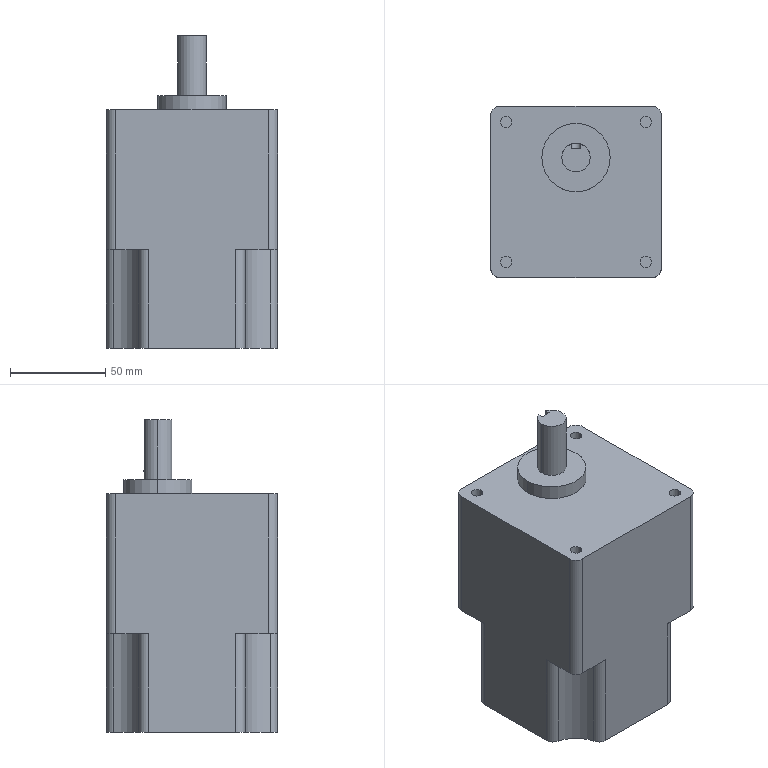Part | SolidWorks | features BaseBody 1 | 1 solid | 48 faces | box 90 x 90 x 164.5 mm | volume 974524 mm3 | cylinder 29 | plane 19 | commonest cylinder face diameters 10 x12 6 x8 35 x4 15 x2 36 x2 5 x1
STEP:
#1=CARTESIAN_POINT('',(-18.,18.,125.5));
#2=VERTEX_POINT('',#1);
#3=CARTESIAN_POINT('',(18.,18.,125.5));
#4=VERTEX_POINT('',#3);
#5=CARTESIAN_POINT('',(0.,18.,125.5));
#6=DIRECTION('',(0.,0.,-1.));
#7=DIRECTION('',(1.,0.,0.));
#8=AXIS2_PLACEMENT_3D('',#5,#6,#7);
#9=CIRCLE('',#8,18.);
#10=EDGE_CURVE('',#2,#4,#9,.T.);
#11=ORIENTED_EDGE('',*,*,#10,.F.);
#12=CARTESIAN_POINT('',(-18.,18.,133.));
#13=VERTEX_POINT('',#12);
#14=CARTESIAN_POINT('',(-18.,18.,125.5));
#15=DIRECTION('',(0.,0.,1.));
#16=VECTOR('',#15,1000.);
#17=LINE('',#14,#16);
#18=EDGE_CURVE('',#2,#13,#17,.T.);
#19=ORIENTED_EDGE('',*,*,#18,.T.);
#20=CARTESIAN_POINT('',(18.,18.,133.));
#21=VERTEX_POINT('',#20);
#22=CARTESIAN_POINT('',(0.,18.,133.));
#23=DIRECTION('',(0.,0.,-1.));
#24=DIRECTION('',(1.,0.,0.));
#25=AXIS2_PLACEMENT_3D('',#22,#23,#24);
#26=CIRCLE('',#25,18.);
#27=EDGE_CURVE('',#13,#21,#26,.T.);
#28=ORIENTED_EDGE('',*,*,#27,.T.);
#29=CARTESIAN_POINT('',(18.,18.,125.5));
#30=DIRECTION('',(0.,0.,1.));
#31=VECTOR('',#30,1000.);
#32=LINE('',#29,#31);
#33=EDGE_CURVE('',#4,#21,#32,.T.);
#34=ORIENTED_EDGE('',*,*,#33,.F.);
#35=EDGE_LOOP('',(#11,#19,#28,#34));
#36=FACE_OUTER_BOUND('',#35,.T.);
#37=CARTESIAN_POINT('',(0.,18.,125.5));
#38=DIRECTION('',(0.,0.,1.));
#39=DIRECTION('',(1.,0.,0.));
#40=AXIS2_PLACEMENT_3D('',#37,#38,#39);
#41=CYLINDRICAL_SURFACE('',#40,18.);
#42=ADVANCED_FACE('',(#36),#41,.T.);
#43=CARTESIAN_POINT('',(-39.77,36.77,110.5));
#44=VERTEX_POINT('',#43);
#45=CARTESIAN_POINT('',(-33.77,36.77,110.5));
#46=VERTEX_POINT('',#45);
#47=CARTESIAN_POINT('',(-36.77,36.77,110.5));
#48=DIRECTION('',(0.,0.,1.));
#49=DIRECTION('',(1.,0.,0.));
#50=AXIS2_PLACEMENT_3D('',#47,#48,#49);
#51=CIRCLE('',#50,3.);
#52=EDGE_CURVE('',#44,#46,#51,.T.);
#53=ORIENTED_EDGE('',*,*,#52,.F.);
#54=CARTESIAN_POINT('',(-39.77,36.77,125.5));
#55=VERTEX_POINT('',#54);
#56=CARTESIAN_POINT('',(-39.77,36.77,125.5));
#57=DIRECTION('',(0.,0.,1.));
#58=VECTOR('',#57,1000.);
#59=LINE('',#56,#58);
#60=EDGE_CURVE('',#44,#55,#59,.T.);
#61=ORIENTED_EDGE('',*,*,#60,.T.);
#62=CARTESIAN_POINT('',(-33.77,36.77,125.5));
#63=VERTEX_POINT('',#62);
#64=CARTESIAN_POINT('',(-36.77,36.77,125.5));
#65=DIRECTION('',(0.,0.,-1.));
#66=DIRECTION('',(1.,0.,0.));
#67=AXIS2_PLACEMENT_3D('',#64,#65,#66);
#68=CIRCLE('',#67,3.);
#69=EDGE_CURVE('',#63,#55,#68,.T.);
#70=ORIENTED_EDGE('',*,*,#69,.F.);
#71=CARTESIAN_POINT('',(-33.77,36.77,125.5));
#72=DIRECTION('',(0.,0.,1.));
#73=VECTOR('',#72,1000.);
#74=LINE('',#71,#73);
#75=EDGE_CURVE('',#46,#63,#74,.T.);
#76=ORIENTED_EDGE('',*,*,#75,.F.);
#77=EDGE_LOOP('',(#53,#61,#70,#76));
#78=FACE_OUTER_BOUND('',#77,.T.);
#79=CARTESIAN_POINT('',(-36.77,36.77,125.5));
#80=DIRECTION('',(0.,0.,1.));
#81=DIRECTION('',(1.,0.,0.));
#82=AXIS2_PLACEMENT_3D('',#79,#80,#81);
#83=CYLINDRICAL_SURFACE('',#82,3.);
#84=ADVANCED_FACE('',(#78),#83,.F.);
#85=CARTESIAN_POINT('',(33.77,36.77,110.5));
#86=VERTEX_POINT('',#85);
#87=CARTESIAN_POINT('',(39.77,36.77,110.5));
#88=VERTEX_POINT('',#87);
#89=CARTESIAN_POINT('',(36.77,36.77,110.5));
#90=DIRECTION('',(0.,0.,1.));
#91=DIRECTION('',(1.,0.,0.));
#92=AXIS2_PLACEMENT_3D('',#89,#90,#91);
#93=CIRCLE('',#92,3.);
#94=EDGE_CURVE('',#86,#88,#93,.T.);
#95=ORIENTED_EDGE('',*,*,#94,.F.);
#96=CARTESIAN_POINT('',(33.77,36.77,125.5));
#97=VERTEX_POINT('',#96);
#98=CARTESIAN_POINT('',(33.77,36.77,125.5));
#99=DIRECTION('',(0.,0.,1.));
#100=VECTOR('',#99,1000.);
#101=LINE('',#98,#100);
#102=EDGE_CURVE('',#86,#97,#101,.T.);
#103=ORIENTED_EDGE('',*,*,#102,.T.);
#104=CARTESIAN_POINT('',(39.77,36.77,125.5));
#105=VERTEX_POINT('',#104);
#106=CARTESIAN_POINT('',(36.77,36.77,125.5));
#107=DIRECTION('',(0.,0.,-1.));
#108=DIRECTION('',(1.,0.,0.));
#109=AXIS2_PLACEMENT_3D('',#106,#107,#108);
#110=CIRCLE('',#109,3.);
#111=EDGE_CURVE('',#105,#97,#110,.T.);
#112=ORIENTED_EDGE('',*,*,#111,.F.);
#113=CARTESIAN_POINT('',(39.77,36.77,125.5));
#114=DIRECTION('',(0.,0.,1.));
#115=VECTOR('',#114,1000.);
#116=LINE('',#113,#115);
#117=EDGE_CURVE('',#88,#105,#116,.T.);
#118=ORIENTED_EDGE('',*,*,#117,.F.);
#119=EDGE_LOOP('',(#95,#103,#112,#118));
#120=FACE_OUTER_BOUND('',#119,.T.);
#121=CARTESIAN_POINT('',(36.77,36.77,125.5));
#122=DIRECTION('',(0.,0.,1.));
#123=DIRECTION('',(1.,0.,0.));
#124=AXIS2_PLACEMENT_3D('',#121,#122,#123);
#125=CYLINDRICAL_SURFACE('',#124,3.);
#126=ADVANCED_FACE('',(#120),#125,.F.);
#127=CARTESIAN_POINT('',(33.77,-36.77,110.5));
#128=VERTEX_POINT('',#127);
#129=CARTESIAN_POINT('',(39.77,-36.77,110.5));
#130=VERTEX_POINT('',#129);
#131=CARTESIAN_POINT('',(36.77,-36.77,110.5));
#132=DIRECTION('',(0.,0.,1.));
#133=DIRECTION('',(1.,0.,0.));
#134=AXIS2_PLACEMENT_3D('',#131,#132,#133);
#135=CIRCLE('',#134,3.);
#136=EDGE_CURVE('',#128,#130,#135,.T.);
#137=ORIENTED_EDGE('',*,*,#136,.F.);
#138=CARTESIAN_POINT('',(33.77,-36.77,125.5));
#139=VERTEX_POINT('',#138);
#140=CARTESIAN_POINT('',(33.77,-36.77,125.5));
#141=DIRECTION('',(0.,0.,1.));
#142=VECTOR('',#141,1000.);
#143=LINE('',#140,#142);
#144=EDGE_CURVE('',#128,#139,#143,.T.);
#145=ORIENTED_EDGE('',*,*,#144,.T.);
#146=CARTESIAN_POINT('',(39.77,-36.77,125.5));
#147=VERTEX_POINT('',#146);
#148=CARTESIAN_POINT('',(36.77,-36.77,125.5));
#149=DIRECTION('',(0.,0.,-1.));
#150=DIRECTION('',(1.,0.,0.));
#151=AXIS2_PLACEMENT_3D('',#148,#149,#150);
#152=CIRCLE('',#151,3.);
#153=EDGE_CURVE('',#147,#139,#152,.T.);
#154=ORIENTED_EDGE('',*,*,#153,.F.);
#155=CARTESIAN_POINT('',(39.77,-36.77,125.5));
#156=DIRECTION('',(0.,0.,1.));
#157=VECTOR('',#156,1000.);
#158=LINE('',#155,#157);
#159=EDGE_CURVE('',#130,#147,#158,.T.);
#160=ORIENTED_EDGE('',*,*,#159,.F.);
#161=EDGE_LOOP('',(#137,#145,#154,#160));
#162=FACE_OUTER_BOUND('',#161,.T.);
#163=CARTESIAN_POINT('',(36.77,-36.77,125.5));
#164=DIRECTION('',(0.,0.,1.));
#165=DIRECTION('',(1.,0.,0.));
#166=AXIS2_PLACEMENT_3D('',#163,#164,#165);
#167=CYLINDRICAL_SURFACE('',#166,3.);
#168=ADVANCED_FACE('',(#162),#167,.F.);
#169=CARTESIAN_POINT('',(-39.77,-36.77,110.5));
#170=VERTEX_POINT('',#169);
#171=CARTESIAN_POINT('',(-33.77,-36.77,110.5));
#172=VERTEX_POINT('',#171);
#173=CARTESIAN_POINT('',(-36.77,-36.77,110.5));
#174=DIRECTION('',(0.,0.,1.));
#175=DIRECTION('',(1.,0.,0.));
#176=AXIS2_PLACEMENT_3D('',#173,#174,#175);
#177=CIRCLE('',#176,3.);
#178=EDGE_CURVE('',#170,#172,#177,.T.);
#179=ORIENTED_EDGE('',*,*,#178,.F.);
#180=CARTESIAN_POINT('',(-39.77,-36.77,125.5));
#181=VERTEX_POINT('',#180);
#182=CARTESIAN_POINT('',(-39.77,-36.77,125.5));
#183=DIRECTION('',(0.,0.,1.));
#184=VECTOR('',#183,1000.);
#185=LINE('',#182,#184);
#186=EDGE_CURVE('',#170,#181,#185,.T.);
#187=ORIENTED_EDGE('',*,*,#186,.T.);
#188=CARTESIAN_POINT('',(-33.77,-36.77,125.5));
#189=VERTEX_POINT('',#188);
#190=CARTESIAN_POINT('',(-36.77,-36.77,125.5));
#191=DIRECTION('',(0.,0.,-1.));
#192=DIRECTION('',(1.,0.,0.));
#193=AXIS2_PLACEMENT_3D('',#190,#191,#192);
#194=CIRCLE('',#193,3.);
#195=EDGE_CURVE('',#189,#181,#194,.T.);
#196=ORIENTED_EDGE('',*,*,#195,.F.);
#197=CARTESIAN_POINT('',(-33.77,-36.77,125.5));
#198=DIRECTION('',(0.,0.,1.));
#199=VECTOR('',#198,1000.);
#200=LINE('',#197,#199);
#201=EDGE_CURVE('',#172,#189,#200,.T.);
#202=ORIENTED_EDGE('',*,*,#201,.F.);
#203=EDGE_LOOP('',(#179,#187,#196,#202));
#204=FACE_OUTER_BOUND('',#203,.T.);
#205=CARTESIAN_POINT('',(-36.77,-36.77,125.5));
#206=DIRECTION('',(0.,0.,1.));
#207=DIRECTION('',(1.,0.,0.));
#208=AXIS2_PLACEMENT_3D('',#205,#206,#207);
#209=CYLINDRICAL_SURFACE('',#208,3.);
#210=ADVANCED_FACE('',(#204),#209,.F.);
#211=CARTESIAN_POINT('',(-7.5,18.,133.));
#212=VERTEX_POINT('',#211);
#213=CARTESIAN_POINT('',(7.5,18.,133.));
#214=VERTEX_POINT('',#213);
#215=CARTESIAN_POINT('',(0.,18.,133.));
#216=DIRECTION('',(0.,0.,-1.));
#217=DIRECTION('',(1.,0.,0.));
#218=AXIS2_PLACEMENT_3D('',#215,#216,#217);
#219=CIRCLE('',#218,7.5);
#220=EDGE_CURVE('',#212,#214,#219,.T.);
#221=ORIENTED_EDGE('',*,*,#220,.F.);
#222=CARTESIAN_POINT('',(-7.5,18.,164.5));
#223=VERTEX_POINT('',#222);
#224=CARTESIAN_POINT('',(-7.5,18.,133.));
#225=DIRECTION('',(0.,0.,1.));
#226=VECTOR('',#225,1000.);
#227=LINE('',#224,#226);
#228=EDGE_CURVE('',#212,#223,#227,.T.);
#229=ORIENTED_EDGE('',*,*,#228,.T.);
#230=CARTESIAN_POINT('',(-2.5,25.071,164.5));
#231=VERTEX_POINT('',#230);
#232=CARTESIAN_POINT('',(0.,18.,164.5));
#233=DIRECTION('',(0.,0.,-1.));
#234=DIRECTION('',(1.,0.,0.));
#235=AXIS2_PLACEMENT_3D('',#232,#233,#234);
#236=CIRCLE('',#235,7.5);
#237=EDGE_CURVE('',#223,#231,#236,.T.);
#238=ORIENTED_EDGE('',*,*,#237,.T.);
#239=CARTESIAN_POINT('',(-2.5,25.071,139.5));
#240=VERTEX_POINT('',#239);
#241=CARTESIAN_POINT('',(-2.5,25.071,133.));
#242=DIRECTION('',(0.,0.,-1.));
#243=VECTOR('',#242,1000.);
#244=LINE('',#241,#243);
#245=EDGE_CURVE('',#231,#240,#244,.T.);
#246=ORIENTED_EDGE('',*,*,#245,.T.);
#247=CARTESIAN_POINT('',(2.5,25.071,139.5));
#248=VERTEX_POINT('',#247);
#249=CARTESIAN_POINT('',(-2.5,25.071,139.5));
#250=CARTESIAN_POINT('',(-2.5,25.071,139.334));
#251=CARTESIAN_POINT('',(-2.484,25.077,139.17));
#252=CARTESIAN_POINT('',(-2.419,25.099,138.849));
#253=CARTESIAN_POINT('',(-2.371,25.116,138.69));
#254=CARTESIAN_POINT('',(-2.245,25.156,138.388));
#255=CARTESIAN_POINT('',(-2.168,25.18,138.245));
#256=CARTESIAN_POINT('',(-1.987,25.233,137.974));
#257=CARTESIAN_POINT('',(-1.883,25.261,137.847));
#258=CARTESIAN_POINT('',(-1.54,25.344,137.504));
#259=CARTESIAN_POINT('',(-1.263,25.399,137.318));
#260=CARTESIAN_POINT('',(-0.8128,25.457,137.13));
#261=CARTESIAN_POINT('',(-0.6543,25.473,137.082));
#262=CARTESIAN_POINT('',(-0.3305,25.494,137.016));
#263=CARTESIAN_POINT('',(-0.1663,25.5,137.));
#264=CARTESIAN_POINT('',(0.1664,25.5,137.));
#265=CARTESIAN_POINT('',(0.3297,25.494,137.016));
#266=CARTESIAN_POINT('',(0.6507,25.473,137.081));
#267=CARTESIAN_POINT('',(0.8101,25.458,137.129));
#268=CARTESIAN_POINT('',(1.112,25.419,137.255));
#269=CARTESIAN_POINT('',(1.255,25.395,137.332));
#270=CARTESIAN_POINT('',(1.526,25.344,137.513));
#271=CARTESIAN_POINT('',(1.653,25.316,137.618));
#272=CARTESIAN_POINT('',(1.996,25.233,137.961));
#273=CARTESIAN_POINT('',(2.182,25.177,138.237));
#274=CARTESIAN_POINT('',(2.37,25.116,138.687));
#275=CARTESIAN_POINT('',(2.419,25.099,138.846));
#276=CARTESIAN_POINT('',(2.484,25.077,139.17));
#277=CARTESIAN_POINT('',(2.5,25.071,139.334));
#278=CARTESIAN_POINT('',(2.5,25.071,139.5));
#279=B_SPLINE_CURVE_WITH_KNOTS('',3,(#249,#250,#251,#252,#253,#254,#255,#256,#257,#258,#259,#260,#261,#262,#263,#264,#265,#266,#267,#268,#269,#270,#271,#272,#273,#274,#275,#276,#277,#278),.UNSPECIFIED.,.F.,.F.,(4,2,2,2,2,2,2,2,2,2,2,2,2,2,4),(-0.003934,-0.003442,-0.00295,-0.002459,-0.001967,-0.0009835,-0.0004917,0.000000013,0.0004917,0.0009835,0.001475,0.001967,0.00295,0.003442,0.003934),.UNSPECIFIED.);
#280=EDGE_CURVE('',#240,#248,#279,.T.);
#281=ORIENTED_EDGE('',*,*,#280,.T.);
#282=CARTESIAN_POINT('',(2.5,25.071,164.5));
#283=VERTEX_POINT('',#282);
#284=CARTESIAN_POINT('',(2.5,25.071,133.));
#285=DIRECTION('',(0.,0.,1.));
#286=VECTOR('',#285,1000.);
#287=LINE('',#284,#286);
#288=EDGE_CURVE('',#248,#283,#287,.T.);
#289=ORIENTED_EDGE('',*,*,#288,.T.);
#290=CARTESIAN_POINT('',(7.5,18.,164.5));
#291=VERTEX_POINT('',#290);
#292=CARTESIAN_POINT('',(0.,18.,164.5));
#293=DIRECTION('',(0.,0.,-1.));
#294=DIRECTION('',(1.,0.,0.));
#295=AXIS2_PLACEMENT_3D('',#292,#293,#294);
#296=CIRCLE('',#295,7.5);
#297=EDGE_CURVE('',#283,#291,#296,.T.);
#298=ORIENTED_EDGE('',*,*,#297,.T.);
#299=CARTESIAN_POINT('',(7.5,18.,133.));
#300=DIRECTION('',(0.,0.,1.));
#301=VECTOR('',#300,1000.);
#302=LINE('',#299,#301);
#303=EDGE_CURVE('',#214,#291,#302,.T.);
#304=ORIENTED_EDGE('',*,*,#303,.F.);
#305=EDGE_LOOP('',(#221,#229,#238,#246,#281,#289,#298,#304));
#306=FACE_OUTER_BOUND('',#305,.T.);
#307=CARTESIAN_POINT('',(0.,18.,133.));
#308=DIRECTION('',(0.,0.,1.));
#309=DIRECTION('',(1.,0.,0.));
#310=AXIS2_PLACEMENT_3D('',#307,#308,#309);
#311=CYLINDRICAL_SURFACE('',#310,7.5);
#312=ADVANCED_FACE('',(#306),#311,.T.);
#313=CARTESIAN_POINT('',(45.,-23.063,0.));
#314=VERTEX_POINT('',#313);
#315=CARTESIAN_POINT('',(45.,23.063,0.));
#316=VERTEX_POINT('',#315);
#317=CARTESIAN_POINT('',(45.,-45.,0.));
#318=DIRECTION('',(0.,1.,0.));
#319=VECTOR('',#318,1000.);
#320=LINE('',#317,#319);
#321=EDGE_CURVE('',#314,#316,#320,.T.);
#322=ORIENTED_EDGE('',*,*,#321,.T.);
#323=CARTESIAN_POINT('',(45.,23.063,52.));
#324=VERTEX_POINT('',#323);
#325=CARTESIAN_POINT('',(45.,23.063,0.));
#326=DIRECTION('',(0.,0.,1.));
#327=VECTOR('',#326,1000.);
#328=LINE('',#325,#327);
#329=EDGE_CURVE('',#316,#324,#328,.T.);
#330=ORIENTED_EDGE('',*,*,#329,.T.);
#331=CARTESIAN_POINT('',(45.,40.,52.));
#332=VERTEX_POINT('',#331);
#333=CARTESIAN_POINT('',(45.,-45.,52.));
#334=DIRECTION('',(0.,1.,0.));
#335=VECTOR('',#334,1000.);
#336=LINE('',#333,#335);
#337=EDGE_CURVE('',#324,#332,#336,.T.);
#338=ORIENTED_EDGE('',*,*,#337,.T.);
#339=CARTESIAN_POINT('',(45.,40.,125.5));
#340=VERTEX_POINT('',#339);
#341=CARTESIAN_POINT('',(45.,40.,0.));
#342=DIRECTION('',(0.,0.,1.));
#343=VECTOR('',#342,1000.);
#344=LINE('',#341,#343);
#345=EDGE_CURVE('',#332,#340,#344,.T.);
#346=ORIENTED_EDGE('',*,*,#345,.T.);
#347=CARTESIAN_POINT('',(45.,-40.,125.5));
#348=VERTEX_POINT('',#347);
#349=CARTESIAN_POINT('',(45.,-45.,125.5));
#350=DIRECTION('',(0.,-1.,0.));
#351=VECTOR('',#350,1000.);
#352=LINE('',#349,#351);
#353=EDGE_CURVE('',#340,#348,#352,.T.);
#354=ORIENTED_EDGE('',*,*,#353,.T.);
#355=CARTESIAN_POINT('',(45.,-40.,52.));
#356=VERTEX_POINT('',#355);
#357=CARTESIAN_POINT('',(45.,-40.,0.));
#358=DIRECTION('',(0.,0.,-1.));
#359=VECTOR('',#358,1000.);
#360=LINE('',#357,#359);
#361=EDGE_CURVE('',#348,#356,#360,.T.);
#362=ORIENTED_EDGE('',*,*,#361,.T.);
#363=CARTESIAN_POINT('',(45.,-23.063,52.));
#364=VERTEX_POINT('',#363);
#365=CARTESIAN_POINT('',(45.,-45.,52.));
#366=DIRECTION('',(0.,1.,0.));
#367=VECTOR('',#366,1000.);
#368=LINE('',#365,#367);
#369=EDGE_CURVE('',#356,#364,#368,.T.);
#370=ORIENTED_EDGE('',*,*,#369,.T.);
#371=CARTESIAN_POINT('',(45.,-23.063,0.));
#372=DIRECTION('',(0.,0.,-1.));
#373=VECTOR('',#372,1000.);
#374=LINE('',#371,#373);
#375=EDGE_CURVE('',#364,#314,#374,.T.);
#376=ORIENTED_EDGE('',*,*,#375,.T.);
#377=EDGE_LOOP('',(#322,#330,#338,#346,#354,#362,#370,#376));
#378=FACE_OUTER_BOUND('',#377,.T.);
#379=CARTESIAN_POINT('',(45.,-45.,0.));
#380=DIRECTION('',(1.,0.,0.));
#381=DIRECTION('',(0.,0.,-1.));
#382=AXIS2_PLACEMENT_3D('',#379,#380,#381);
#383=PLANE('',#382);
#384=ADVANCED_FACE('',(#378),#383,.T.);
#385=CARTESIAN_POINT('',(41.111,27.938,0.));
#386=VERTEX_POINT('',#385);
#387=CARTESIAN_POINT('',(40.,23.063,0.));
#388=DIRECTION('',(0.,0.,1.));
#389=DIRECTION('',(1.,0.,0.));
#390=AXIS2_PLACEMENT_3D('',#387,#388,#389);
#391=CIRCLE('',#390,5.);
#392=EDGE_CURVE('',#316,#386,#391,.T.);
#393=ORIENTED_EDGE('',*,*,#392,.T.);
#394=CARTESIAN_POINT('',(41.111,27.938,52.));
#395=VERTEX_POINT('',#394);
#396=CARTESIAN_POINT('',(41.111,27.938,-214.442));
#397=DIRECTION('',(0.,0.,1.));
#398=VECTOR('',#397,1000.);
#399=LINE('',#396,#398);
#400=EDGE_CURVE('',#386,#395,#399,.T.);
#401=ORIENTED_EDGE('',*,*,#400,.T.);
#402=CARTESIAN_POINT('',(40.,23.063,52.));
#403=DIRECTION('',(0.,0.,-1.));
#404=DIRECTION('',(1.,0.,0.));
#405=AXIS2_PLACEMENT_3D('',#402,#403,#404);
#406=CIRCLE('',#405,5.);
#407=EDGE_CURVE('',#395,#324,#406,.T.);
#408=ORIENTED_EDGE('',*,*,#407,.T.);
#409=ORIENTED_EDGE('',*,*,#329,.F.);
#410=EDGE_LOOP('',(#393,#401,#408,#409));
#411=FACE_OUTER_BOUND('',#410,.T.);
#412=CARTESIAN_POINT('',(40.,23.063,-214.442));
#413=DIRECTION('',(0.,0.,1.));
#414=DIRECTION('',(1.,0.,0.));
#415=AXIS2_PLACEMENT_3D('',#412,#413,#414);
#416=CYLINDRICAL_SURFACE('',#415,5.);
#417=ADVANCED_FACE('',(#411),#416,.T.);
#418=CARTESIAN_POINT('',(41.111,-27.938,0.));
#419=VERTEX_POINT('',#418);
#420=CARTESIAN_POINT('',(40.,-23.063,0.));
#421=DIRECTION('',(0.,0.,1.));
#422=DIRECTION('',(-1.,0.,0.));
#423=AXIS2_PLACEMENT_3D('',#420,#421,#422);
#424=CIRCLE('',#423,5.);
#425=EDGE_CURVE('',#419,#314,#424,.T.);
#426=ORIENTED_EDGE('',*,*,#425,.F.);
#427=CARTESIAN_POINT('',(27.938,-41.111,0.));
#428=VERTEX_POINT('',#427);
#429=CARTESIAN_POINT('',(45.,-45.,0.));
#430=DIRECTION('',(0.,0.,-1.));
#431=DIRECTION('',(-1.,0.,0.));
#432=AXIS2_PLACEMENT_3D('',#429,#430,#431);
#433=CIRCLE('',#432,17.5);
#434=EDGE_CURVE('',#428,#419,#433,.T.);
#435=ORIENTED_EDGE('',*,*,#434,.F.);
#436=CARTESIAN_POINT('',(23.063,-45.,0.));
#437=VERTEX_POINT('',#436);
#438=CARTESIAN_POINT('',(23.063,-40.,0.));
#439=DIRECTION('',(0.,0.,1.));
#440=DIRECTION('',(1.,0.,0.));
#441=AXIS2_PLACEMENT_3D('',#438,#439,#440);
#442=CIRCLE('',#441,5.);
#443=EDGE_CURVE('',#437,#428,#442,.T.);
#444=ORIENTED_EDGE('',*,*,#443,.F.);
#445=CARTESIAN_POINT('',(-23.063,-45.,0.));
#446=VERTEX_POINT('',#445);
#447=CARTESIAN_POINT('',(0.,-45.,0.));
#448=DIRECTION('',(1.,0.,0.));
#449=VECTOR('',#448,1000.);
#450=LINE('',#447,#449);
#451=EDGE_CURVE('',#446,#437,#450,.T.);
#452=ORIENTED_EDGE('',*,*,#451,.F.);
#453=CARTESIAN_POINT('',(-27.938,-41.111,0.));
#454=VERTEX_POINT('',#453);
#455=CARTESIAN_POINT('',(-23.063,-40.,0.));
#456=DIRECTION('',(0.,0.,1.));
#457=DIRECTION('',(-1.,0.,0.));
#458=AXIS2_PLACEMENT_3D('',#455,#456,#457);
#459=CIRCLE('',#458,5.);
#460=EDGE_CURVE('',#454,#446,#459,.T.);
#461=ORIENTED_EDGE('',*,*,#460,.F.);
#462=CARTESIAN_POINT('',(-41.111,-27.938,0.));
#463=VERTEX_POINT('',#462);
#464=CARTESIAN_POINT('',(-45.,-45.,0.));
#465=DIRECTION('',(0.,0.,-1.));
#466=DIRECTION('',(-1.,0.,0.));
#467=AXIS2_PLACEMENT_3D('',#464,#465,#466);
#468=CIRCLE('',#467,17.5);
#469=EDGE_CURVE('',#463,#454,#468,.T.);
#470=ORIENTED_EDGE('',*,*,#469,.F.);
#471=CARTESIAN_POINT('',(-45.,-23.063,0.));
#472=VERTEX_POINT('',#471);
#473=CARTESIAN_POINT('',(-40.,-23.063,0.));
#474=DIRECTION('',(0.,0.,1.));
#475=DIRECTION('',(1.,0.,0.));
#476=AXIS2_PLACEMENT_3D('',#473,#474,#475);
#477=CIRCLE('',#476,5.);
#478=EDGE_CURVE('',#472,#463,#477,.T.);
#479=ORIENTED_EDGE('',*,*,#478,.F.);
#480=CARTESIAN_POINT('',(-45.,23.063,0.));
#481=VERTEX_POINT('',#480);
#482=CARTESIAN_POINT('',(-45.,0.,0.));
#483=DIRECTION('',(0.,-1.,0.));
#484=VECTOR('',#483,1000.);
#485=LINE('',#482,#484);
#486=EDGE_CURVE('',#481,#472,#485,.T.);
#487=ORIENTED_EDGE('',*,*,#486,.F.);
#488=CARTESIAN_POINT('',(-41.111,27.938,0.));
#489=VERTEX_POINT('',#488);
#490=CARTESIAN_POINT('',(-40.,23.063,0.));
#491=DIRECTION('',(0.,0.,1.));
#492=DIRECTION('',(-1.,0.,0.));
#493=AXIS2_PLACEMENT_3D('',#490,#491,#492);
#494=CIRCLE('',#493,5.);
#495=EDGE_CURVE('',#489,#481,#494,.T.);
#496=ORIENTED_EDGE('',*,*,#495,.F.);
#497=CARTESIAN_POINT('',(-27.938,41.111,0.));
#498=VERTEX_POINT('',#497);
#499=CARTESIAN_POINT('',(-45.,45.,0.));
#500=DIRECTION('',(0.,0.,-1.));
#501=DIRECTION('',(-1.,0.,0.));
#502=AXIS2_PLACEMENT_3D('',#499,#500,#501);
#503=CIRCLE('',#502,17.5);
#504=EDGE_CURVE('',#498,#489,#503,.T.);
#505=ORIENTED_EDGE('',*,*,#504,.F.);
#506=CARTESIAN_POINT('',(-23.063,45.,0.));
#507=VERTEX_POINT('',#506);
#508=CARTESIAN_POINT('',(-23.063,40.,0.));
#509=DIRECTION('',(0.,0.,1.));
#510=DIRECTION('',(1.,0.,0.));
#511=AXIS2_PLACEMENT_3D('',#508,#509,#510);
#512=CIRCLE('',#511,5.);
#513=EDGE_CURVE('',#507,#498,#512,.T.);
#514=ORIENTED_EDGE('',*,*,#513,.F.);
#515=CARTESIAN_POINT('',(23.063,45.,0.));
#516=VERTEX_POINT('',#515);
#517=CARTESIAN_POINT('',(0.,45.,0.));
#518=DIRECTION('',(-1.,0.,0.));
#519=VECTOR('',#518,1000.);
#520=LINE('',#517,#519);
#521=EDGE_CURVE('',#516,#507,#520,.T.);
#522=ORIENTED_EDGE('',*,*,#521,.F.);
#523=CARTESIAN_POINT('',(27.938,41.111,0.));
#524=VERTEX_POINT('',#523);
#525=CARTESIAN_POINT('',(23.063,40.,0.));
#526=DIRECTION('',(0.,0.,1.));
#527=DIRECTION('',(-1.,0.,0.));
#528=AXIS2_PLACEMENT_3D('',#525,#526,#527);
#529=CIRCLE('',#528,5.);
#530=EDGE_CURVE('',#524,#516,#529,.T.);
#531=ORIENTED_EDGE('',*,*,#530,.F.);
#532=CARTESIAN_POINT('',(45.,45.,0.));
#533=DIRECTION('',(0.,0.,-1.));
#534=DIRECTION('',(-1.,0.,0.));
#535=AXIS2_PLACEMENT_3D('',#532,#533,#534);
#536=CIRCLE('',#535,17.5);
#537=EDGE_CURVE('',#386,#524,#536,.T.);
#538=ORIENTED_EDGE('',*,*,#537,.F.);
#539=ORIENTED_EDGE('',*,*,#392,.F.);
#540=ORIENTED_EDGE('',*,*,#321,.F.);
#541=EDGE_LOOP('',(#426,#435,#444,#452,#461,#470,#479,#487,#496,#505,#514,#522,#531,#538,#539,#540));
#542=FACE_OUTER_BOUND('',#541,.T.);
#543=CARTESIAN_POINT('',(0.,0.,0.));
#544=DIRECTION('',(0.,0.,1.));
#545=DIRECTION('',(1.,0.,0.));
#546=AXIS2_PLACEMENT_3D('',#543,#544,#545);
#547=PLANE('',#546);
#548=ADVANCED_FACE('',(#542),#547,.F.);
#549=CARTESIAN_POINT('',(41.111,-27.938,52.));
#550=VERTEX_POINT('',#549);
#551=CARTESIAN_POINT('',(41.111,-27.938,378.942));
#552=DIRECTION('',(0.,0.,-1.));
#553=VECTOR('',#552,1000.);
#554=LINE('',#551,#553);
#555=EDGE_CURVE('',#550,#419,#554,.T.);
#556=ORIENTED_EDGE('',*,*,#555,.T.);
#557=ORIENTED_EDGE('',*,*,#425,.T.);
#558=ORIENTED_EDGE('',*,*,#375,.F.);
#559=CARTESIAN_POINT('',(40.,-23.063,52.));
#560=DIRECTION('',(0.,0.,-1.));
#561=DIRECTION('',(-1.,0.,0.));
#562=AXIS2_PLACEMENT_3D('',#559,#560,#561);
#563=CIRCLE('',#562,5.);
#564=EDGE_CURVE('',#364,#550,#563,.T.);
#565=ORIENTED_EDGE('',*,*,#564,.T.);
#566=EDGE_LOOP('',(#556,#557,#558,#565));
#567=FACE_OUTER_BOUND('',#566,.T.);
#568=CARTESIAN_POINT('',(40.,-23.063,378.942));
#569=DIRECTION('',(0.,0.,-1.));
#570=DIRECTION('',(-1.,0.,0.));
#571=AXIS2_PLACEMENT_3D('',#568,#569,#570);
#572=CYLINDRICAL_SURFACE('',#571,5.);
#573=ADVANCED_FACE('',(#567),#572,.T.);
#574=CARTESIAN_POINT('',(23.063,-45.,52.));
#575=VERTEX_POINT('',#574);
#576=CARTESIAN_POINT('',(27.938,-41.111,52.));
#577=VERTEX_POINT('',#576);
#578=CARTESIAN_POINT('',(23.063,-40.,52.));
#579=DIRECTION('',(0.,0.,1.));
#580=DIRECTION('',(1.,0.,0.));
#581=AXIS2_PLACEMENT_3D('',#578,#579,#580);
#582=CIRCLE('',#581,5.);
#583=EDGE_CURVE('',#575,#577,#582,.T.);
#584=ORIENTED_EDGE('',*,*,#583,.T.);
#585=CARTESIAN_POINT('',(45.,-45.,52.));
#586=DIRECTION('',(0.,0.,-1.));
#587=DIRECTION('',(-1.,0.,0.));
#588=AXIS2_PLACEMENT_3D('',#585,#586,#587);
#589=CIRCLE('',#588,17.5);
#590=EDGE_CURVE('',#577,#550,#589,.T.);
#591=ORIENTED_EDGE('',*,*,#590,.T.);
#592=ORIENTED_EDGE('',*,*,#564,.F.);
#593=ORIENTED_EDGE('',*,*,#369,.F.);
#594=CARTESIAN_POINT('',(40.,-45.,52.));
#595=VERTEX_POINT('',#594);
#596=CARTESIAN_POINT('',(40.,-40.,52.));
#597=DIRECTION('',(0.,0.,-1.));
#598=DIRECTION('',(-1.,0.,0.));
#599=AXIS2_PLACEMENT_3D('',#596,#597,#598);
#600=CIRCLE('',#599,5.);
#601=EDGE_CURVE('',#356,#595,#600,.T.);
#602=ORIENTED_EDGE('',*,*,#601,.T.);
#603=CARTESIAN_POINT('',(0.,-45.,52.));
#604=DIRECTION('',(-1.,0.,0.));
#605=VECTOR('',#604,1000.);
#606=LINE('',#603,#605);
#607=EDGE_CURVE('',#595,#575,#606,.T.);
#608=ORIENTED_EDGE('',*,*,#607,.T.);
#609=EDGE_LOOP('',(#584,#591,#592,#593,#602,#608));
#610=FACE_OUTER_BOUND('',#609,.T.);
#611=CARTESIAN_POINT('',(0.,0.,52.));
#612=DIRECTION('',(0.,0.,-1.));
#613=DIRECTION('',(-1.,0.,0.));
#614=AXIS2_PLACEMENT_3D('',#611,#612,#613);
#615=PLANE('',#614);
#616=ADVANCED_FACE('',(#610),#615,.T.);
#617=CARTESIAN_POINT('',(40.,-45.,125.5));
#618=VERTEX_POINT('',#617);
#619=CARTESIAN_POINT('',(40.,-45.,378.942));
#620=DIRECTION('',(0.,0.,-1.));
#621=VECTOR('',#620,1000.);
#622=LINE('',#619,#621);
#623=EDGE_CURVE('',#618,#595,#622,.T.);
#624=ORIENTED_EDGE('',*,*,#623,.T.);
#625=ORIENTED_EDGE('',*,*,#601,.F.);
#626=ORIENTED_EDGE('',*,*,#361,.F.);
#627=CARTESIAN_POINT('',(40.,-40.,125.5));
#628=DIRECTION('',(0.,0.,-1.));
#629=DIRECTION('',(-1.,0.,0.));
#630=AXIS2_PLACEMENT_3D('',#627,#628,#629);
#631=CIRCLE('',#630,5.);
#632=EDGE_CURVE('',#348,#618,#631,.T.);
#633=ORIENTED_EDGE('',*,*,#632,.T.);
#634=EDGE_LOOP('',(#624,#625,#626,#633));
#635=FACE_OUTER_BOUND('',#634,.T.);
#636=CARTESIAN_POINT('',(40.,-40.,378.942));
#637=DIRECTION('',(0.,0.,-1.));
#638=DIRECTION('',(-1.,0.,0.));
#639=AXIS2_PLACEMENT_3D('',#636,#637,#638);
#640=CYLINDRICAL_SURFACE('',#639,5.);
#641=ADVANCED_FACE('',(#635),#640,.T.);
#642=CARTESIAN_POINT('',(-40.,-45.,125.5));
#643=VERTEX_POINT('',#642);
#644=CARTESIAN_POINT('',(0.,-45.,125.5));
#645=DIRECTION('',(1.,0.,0.));
#646=VECTOR('',#645,1000.);
#647=LINE('',#644,#646);
#648=EDGE_CURVE('',#643,#618,#647,.T.);
#649=ORIENTED_EDGE('',*,*,#648,.T.);
#650=ORIENTED_EDGE('',*,*,#632,.F.);
#651=ORIENTED_EDGE('',*,*,#353,.F.);
#652=CARTESIAN_POINT('',(40.,45.,125.5));
#653=VERTEX_POINT('',#652);
#654=CARTESIAN_POINT('',(40.,40.,125.5));
#655=DIRECTION('',(0.,0.,1.));
#656=DIRECTION('',(-1.,0.,0.));
#657=AXIS2_PLACEMENT_3D('',#654,#655,#656);
#658=CIRCLE('',#657,5.);
#659=EDGE_CURVE('',#340,#653,#658,.T.);
#660=ORIENTED_EDGE('',*,*,#659,.T.);
#661=CARTESIAN_POINT('',(-40.,45.,125.5));
#662=VERTEX_POINT('',#661);
#663=CARTESIAN_POINT('',(0.,45.,125.5));
#664=DIRECTION('',(-1.,0.,0.));
#665=VECTOR('',#664,1000.);
#666=LINE('',#663,#665);
#667=EDGE_CURVE('',#653,#662,#666,.T.);
#668=ORIENTED_EDGE('',*,*,#667,.T.);
#669=CARTESIAN_POINT('',(-45.,40.,125.5));
#670=VERTEX_POINT('',#669);
#671=CARTESIAN_POINT('',(-40.,40.,125.5));
#672=DIRECTION('',(0.,0.,1.));
#673=DIRECTION('',(-1.,0.,0.));
#674=AXIS2_PLACEMENT_3D('',#671,#672,#673);
#675=CIRCLE('',#674,5.);
#676=EDGE_CURVE('',#662,#670,#675,.T.);
#677=ORIENTED_EDGE('',*,*,#676,.T.);
#678=CARTESIAN_POINT('',(-45.,-40.,125.5));
#679=VERTEX_POINT('',#678);
#680=CARTESIAN_POINT('',(-45.,0.,125.5));
#681=DIRECTION('',(0.,-1.,0.));
#682=VECTOR('',#681,1000.);
#683=LINE('',#680,#682);
#684=EDGE_CURVE('',#670,#679,#683,.T.);
#685=ORIENTED_EDGE('',*,*,#684,.T.);
#686=CARTESIAN_POINT('',(-40.,-40.,125.5));
#687=DIRECTION('',(0.,0.,1.));
#688=DIRECTION('',(-1.,0.,0.));
#689=AXIS2_PLACEMENT_3D('',#686,#687,#688);
#690=CIRCLE('',#689,5.);
#691=EDGE_CURVE('',#679,#643,#690,.T.);
#692=ORIENTED_EDGE('',*,*,#691,.T.);
#693=EDGE_LOOP('',(#649,#650,#651,#660,#668,#677,#685,#692));
#694=FACE_OUTER_BOUND('',#693,.T.);
#695=CARTESIAN_POINT('',(0.,18.,125.5));
#696=DIRECTION('',(0.,0.,-1.));
#697=DIRECTION('',(1.,0.,0.));
#698=AXIS2_PLACEMENT_3D('',#695,#696,#697);
#699=CIRCLE('',#698,18.);
#700=EDGE_CURVE('',#4,#2,#699,.T.);
#701=ORIENTED_EDGE('',*,*,#700,.T.);
#702=ORIENTED_EDGE('',*,*,#10,.T.);
#703=EDGE_LOOP('',(#701,#702));
#704=FACE_BOUND('',#703,.T.);
#705=ORIENTED_EDGE('',*,*,#69,.T.);
#706=CARTESIAN_POINT('',(-36.77,36.77,125.5));
#707=DIRECTION('',(0.,0.,-1.));
#708=DIRECTION('',(1.,0.,0.));
#709=AXIS2_PLACEMENT_3D('',#706,#707,#708);
#710=CIRCLE('',#709,3.);
#711=EDGE_CURVE('',#55,#63,#710,.T.);
#712=ORIENTED_EDGE('',*,*,#711,.T.);
#713=EDGE_LOOP('',(#705,#712));
#714=FACE_BOUND('',#713,.T.);
#715=ORIENTED_EDGE('',*,*,#111,.T.);
#716=CARTESIAN_POINT('',(36.77,36.77,125.5));
#717=DIRECTION('',(0.,0.,-1.));
#718=DIRECTION('',(1.,0.,0.));
#719=AXIS2_PLACEMENT_3D('',#716,#717,#718);
#720=CIRCLE('',#719,3.);
#721=EDGE_CURVE('',#97,#105,#720,.T.);
#722=ORIENTED_EDGE('',*,*,#721,.T.);
#723=EDGE_LOOP('',(#715,#722));
#724=FACE_BOUND('',#723,.T.);
#725=ORIENTED_EDGE('',*,*,#153,.T.);
#726=CARTESIAN_POINT('',(36.77,-36.77,125.5));
#727=DIRECTION('',(0.,0.,-1.));
#728=DIRECTION('',(1.,0.,0.));
#729=AXIS2_PLACEMENT_3D('',#726,#727,#728);
#730=CIRCLE('',#729,3.);
#731=EDGE_CURVE('',#139,#147,#730,.T.);
#732=ORIENTED_EDGE('',*,*,#731,.T.);
#733=EDGE_LOOP('',(#725,#732));
#734=FACE_BOUND('',#733,.T.);
#735=ORIENTED_EDGE('',*,*,#195,.T.);
#736=CARTESIAN_POINT('',(-36.77,-36.77,125.5));
#737=DIRECTION('',(0.,0.,-1.));
#738=DIRECTION('',(1.,0.,0.));
#739=AXIS2_PLACEMENT_3D('',#736,#737,#738);
#740=CIRCLE('',#739,3.);
#741=EDGE_CURVE('',#181,#189,#740,.T.);
#742=ORIENTED_EDGE('',*,*,#741,.T.);
#743=EDGE_LOOP('',(#735,#742));
#744=FACE_BOUND('',#743,.T.);
#745=CARTESIAN_POINT('',(0.,0.,125.5));
#746=DIRECTION('',(0.,0.,1.));
#747=DIRECTION('',(1.,0.,0.));
#748=AXIS2_PLACEMENT_3D('',#745,#746,#747);
#749=PLANE('',#748);
#750=ADVANCED_FACE('',(#694,#704,#714,#724,#734,#744),#749,.T.);
#751=ORIENTED_EDGE('',*,*,#345,.F.);
#752=CARTESIAN_POINT('',(40.,45.,52.));
#753=VERTEX_POINT('',#752);
#754=CARTESIAN_POINT('',(40.,40.,52.));
#755=DIRECTION('',(0.,0.,1.));
#756=DIRECTION('',(-1.,0.,0.));
#757=AXIS2_PLACEMENT_3D('',#754,#755,#756);
#758=CIRCLE('',#757,5.);
#759=EDGE_CURVE('',#332,#753,#758,.T.);
#760=ORIENTED_EDGE('',*,*,#759,.T.);
#761=CARTESIAN_POINT('',(40.,45.,378.942));
#762=DIRECTION('',(0.,0.,1.));
#763=VECTOR('',#762,1000.);
#764=LINE('',#761,#763);
#765=EDGE_CURVE('',#753,#653,#764,.T.);
#766=ORIENTED_EDGE('',*,*,#765,.T.);
#767=ORIENTED_EDGE('',*,*,#659,.F.);
#768=EDGE_LOOP('',(#751,#760,#766,#767));
#769=FACE_OUTER_BOUND('',#768,.T.);
#770=CARTESIAN_POINT('',(40.,40.,378.942));
#771=DIRECTION('',(0.,0.,-1.));
#772=DIRECTION('',(-1.,0.,0.));
#773=AXIS2_PLACEMENT_3D('',#770,#771,#772);
#774=CYLINDRICAL_SURFACE('',#773,5.);
#775=ADVANCED_FACE('',(#769),#774,.T.);
#776=CARTESIAN_POINT('',(27.938,41.111,52.));
#777=VERTEX_POINT('',#776);
#778=CARTESIAN_POINT('',(23.063,45.,52.));
#779=VERTEX_POINT('',#778);
#780=CARTESIAN_POINT('',(23.063,40.,52.));
#781=DIRECTION('',(0.,0.,1.));
#782=DIRECTION('',(-1.,0.,0.));
#783=AXIS2_PLACEMENT_3D('',#780,#781,#782);
#784=CIRCLE('',#783,5.);
#785=EDGE_CURVE('',#777,#779,#784,.T.);
#786=ORIENTED_EDGE('',*,*,#785,.T.);
#787=CARTESIAN_POINT('',(0.,45.,52.));
#788=DIRECTION('',(1.,0.,0.));
#789=VECTOR('',#788,1000.);
#790=LINE('',#787,#789);
#791=EDGE_CURVE('',#779,#753,#790,.T.);
#792=ORIENTED_EDGE('',*,*,#791,.T.);
#793=ORIENTED_EDGE('',*,*,#759,.F.);
#794=ORIENTED_EDGE('',*,*,#337,.F.);
#795=ORIENTED_EDGE('',*,*,#407,.F.);
#796=CARTESIAN_POINT('',(45.,45.,52.));
#797=DIRECTION('',(0.,0.,-1.));
#798=DIRECTION('',(-1.,0.,0.));
#799=AXIS2_PLACEMENT_3D('',#796,#797,#798);
#800=CIRCLE('',#799,17.5);
#801=EDGE_CURVE('',#395,#777,#800,.T.);
#802=ORIENTED_EDGE('',*,*,#801,.T.);
#803=EDGE_LOOP('',(#786,#792,#793,#794,#795,#802));
#804=FACE_OUTER_BOUND('',#803,.T.);
#805=CARTESIAN_POINT('',(0.,0.,52.));
#806=DIRECTION('',(0.,0.,-1.));
#807=DIRECTION('',(-1.,0.,0.));
#808=AXIS2_PLACEMENT_3D('',#805,#806,#807);
#809=PLANE('',#808);
#810=ADVANCED_FACE('',(#804),#809,.T.);
#811=CARTESIAN_POINT('',(27.938,41.111,0.));
#812=DIRECTION('',(0.,0.,-1.));
#813=VECTOR('',#812,1000.);
#814=LINE('',#811,#813);
#815=EDGE_CURVE('',#777,#524,#814,.T.);
#816=ORIENTED_EDGE('',*,*,#815,.F.);
#817=ORIENTED_EDGE('',*,*,#801,.F.);
#818=ORIENTED_EDGE('',*,*,#400,.F.);
#819=ORIENTED_EDGE('',*,*,#537,.T.);
#820=EDGE_LOOP('',(#816,#817,#818,#819));
#821=FACE_OUTER_BOUND('',#820,.T.);
#822=CARTESIAN_POINT('',(45.,45.,0.));
#823=DIRECTION('',(0.,0.,-1.));
#824=DIRECTION('',(-1.,0.,0.));
#825=AXIS2_PLACEMENT_3D('',#822,#823,#824);
#826=CYLINDRICAL_SURFACE('',#825,17.5);
#827=ADVANCED_FACE('',(#821),#826,.F.);
#828=ORIENTED_EDGE('',*,*,#555,.F.);
#829=ORIENTED_EDGE('',*,*,#590,.F.);
#830=CARTESIAN_POINT('',(27.938,-41.111,0.));
#831=DIRECTION('',(0.,0.,1.));
#832=VECTOR('',#831,1000.);
#833=LINE('',#830,#832);
#834=EDGE_CURVE('',#428,#577,#833,.T.);
#835=ORIENTED_EDGE('',*,*,#834,.F.);
#836=ORIENTED_EDGE('',*,*,#434,.T.);
#837=EDGE_LOOP('',(#828,#829,#835,#836));
#838=FACE_OUTER_BOUND('',#837,.T.);
#839=CARTESIAN_POINT('',(45.,-45.,0.));
#840=DIRECTION('',(0.,0.,-1.));
#841=DIRECTION('',(-1.,0.,0.));
#842=AXIS2_PLACEMENT_3D('',#839,#840,#841);
#843=CYLINDRICAL_SURFACE('',#842,17.5);
#844=ADVANCED_FACE('',(#838),#843,.F.);
#845=ORIENTED_EDGE('',*,*,#443,.T.);
#846=ORIENTED_EDGE('',*,*,#834,.T.);
#847=ORIENTED_EDGE('',*,*,#583,.F.);
#848=CARTESIAN_POINT('',(23.063,-45.,-214.442));
#849=DIRECTION('',(0.,0.,-1.));
#850=VECTOR('',#849,1000.);
#851=LINE('',#848,#850);
#852=EDGE_CURVE('',#575,#437,#851,.T.);
#853=ORIENTED_EDGE('',*,*,#852,.T.);
#854=EDGE_LOOP('',(#845,#846,#847,#853));
#855=FACE_OUTER_BOUND('',#854,.T.);
#856=CARTESIAN_POINT('',(23.063,-40.,-214.442));
#857=DIRECTION('',(0.,0.,1.));
#858=DIRECTION('',(1.,0.,0.));
#859=AXIS2_PLACEMENT_3D('',#856,#857,#858);
#860=CYLINDRICAL_SURFACE('',#859,5.);
#861=ADVANCED_FACE('',(#855),#860,.T.);
#862=CARTESIAN_POINT('',(-40.,-45.,52.));
#863=VERTEX_POINT('',#862);
#864=CARTESIAN_POINT('',(-23.063,-45.,52.));
#865=VERTEX_POINT('',#864);
#866=CARTESIAN_POINT('',(-45.,-45.,52.));
#867=DIRECTION('',(1.,0.,0.));
#868=VECTOR('',#867,1000.);
#869=LINE('',#866,#868);
#870=EDGE_CURVE('',#863,#865,#869,.T.);
#871=ORIENTED_EDGE('',*,*,#870,.T.);
#872=CARTESIAN_POINT('',(-23.063,-45.,0.));
#873=DIRECTION('',(0.,0.,-1.));
#874=VECTOR('',#873,1000.);
#875=LINE('',#872,#874);
#876=EDGE_CURVE('',#865,#446,#875,.T.);
#877=ORIENTED_EDGE('',*,*,#876,.T.);
#878=ORIENTED_EDGE('',*,*,#451,.T.);
#879=ORIENTED_EDGE('',*,*,#852,.F.);
#880=ORIENTED_EDGE('',*,*,#607,.F.);
#881=ORIENTED_EDGE('',*,*,#623,.F.);
#882=ORIENTED_EDGE('',*,*,#648,.F.);
#883=CARTESIAN_POINT('',(-40.,-45.,0.));
#884=DIRECTION('',(0.,0.,-1.));
#885=VECTOR('',#884,1000.);
#886=LINE('',#883,#885);
#887=EDGE_CURVE('',#643,#863,#886,.T.);
#888=ORIENTED_EDGE('',*,*,#887,.T.);
#889=EDGE_LOOP('',(#871,#877,#878,#879,#880,#881,#882,#888));
#890=FACE_OUTER_BOUND('',#889,.T.);
#891=CARTESIAN_POINT('',(-45.,-45.,0.));
#892=DIRECTION('',(0.,-1.,0.));
#893=DIRECTION('',(0.,0.,-1.));
#894=AXIS2_PLACEMENT_3D('',#891,#892,#893);
#895=PLANE('',#894);
#896=ADVANCED_FACE('',(#890),#895,.T.);
#897=CARTESIAN_POINT('',(-27.938,-41.111,52.));
#898=VERTEX_POINT('',#897);
#899=CARTESIAN_POINT('',(-27.938,-41.111,378.942));
#900=DIRECTION('',(0.,0.,-1.));
#901=VECTOR('',#900,1000.);
#902=LINE('',#899,#901);
#903=EDGE_CURVE('',#898,#454,#902,.T.);
#904=ORIENTED_EDGE('',*,*,#903,.T.);
#905=ORIENTED_EDGE('',*,*,#460,.T.);
#906=ORIENTED_EDGE('',*,*,#876,.F.);
#907=CARTESIAN_POINT('',(-23.063,-40.,52.));
#908=DIRECTION('',(0.,0.,-1.));
#909=DIRECTION('',(-1.,0.,0.));
#910=AXIS2_PLACEMENT_3D('',#907,#908,#909);
#911=CIRCLE('',#910,5.);
#912=EDGE_CURVE('',#865,#898,#911,.T.);
#913=ORIENTED_EDGE('',*,*,#912,.T.);
#914=EDGE_LOOP('',(#904,#905,#906,#913));
#915=FACE_OUTER_BOUND('',#914,.T.);
#916=CARTESIAN_POINT('',(-23.063,-40.,378.942));
#917=DIRECTION('',(0.,0.,-1.));
#918=DIRECTION('',(-1.,0.,0.));
#919=AXIS2_PLACEMENT_3D('',#916,#917,#918);
#920=CYLINDRICAL_SURFACE('',#919,5.);
#921=ADVANCED_FACE('',(#915),#920,.T.);
#922=ORIENTED_EDGE('',*,*,#903,.F.);
#923=CARTESIAN_POINT('',(-41.111,-27.938,52.));
#924=VERTEX_POINT('',#923);
#925=CARTESIAN_POINT('',(-45.,-45.,52.));
#926=DIRECTION('',(0.,0.,-1.));
#927=DIRECTION('',(-1.,0.,0.));
#928=AXIS2_PLACEMENT_3D('',#925,#926,#927);
#929=CIRCLE('',#928,17.5);
#930=EDGE_CURVE('',#924,#898,#929,.T.);
#931=ORIENTED_EDGE('',*,*,#930,.F.);
#932=CARTESIAN_POINT('',(-41.111,-27.938,0.));
#933=DIRECTION('',(0.,0.,1.));
#934=VECTOR('',#933,1000.);
#935=LINE('',#932,#934);
#936=EDGE_CURVE('',#463,#924,#935,.T.);
#937=ORIENTED_EDGE('',*,*,#936,.F.);
#938=ORIENTED_EDGE('',*,*,#469,.T.);
#939=EDGE_LOOP('',(#922,#931,#937,#938));
#940=FACE_OUTER_BOUND('',#939,.T.);
#941=CARTESIAN_POINT('',(-45.,-45.,0.));
#942=DIRECTION('',(0.,0.,-1.));
#943=DIRECTION('',(-1.,0.,0.));
#944=AXIS2_PLACEMENT_3D('',#941,#942,#943);
#945=CYLINDRICAL_SURFACE('',#944,17.5);
#946=ADVANCED_FACE('',(#940),#945,.F.);
#947=ORIENTED_EDGE('',*,*,#478,.T.);
#948=ORIENTED_EDGE('',*,*,#936,.T.);
#949=CARTESIAN_POINT('',(-45.,-23.063,52.));
#950=VERTEX_POINT('',#949);
#951=CARTESIAN_POINT('',(-40.,-23.063,52.));
#952=DIRECTION('',(0.,0.,-1.));
#953=DIRECTION('',(1.,0.,0.));
#954=AXIS2_PLACEMENT_3D('',#951,#952,#953);
#955=CIRCLE('',#954,5.);
#956=EDGE_CURVE('',#924,#950,#955,.T.);
#957=ORIENTED_EDGE('',*,*,#956,.T.);
#958=CARTESIAN_POINT('',(-45.,-23.063,-214.442));
#959=DIRECTION('',(0.,0.,-1.));
#960=VECTOR('',#959,1000.);
#961=LINE('',#958,#960);
#962=EDGE_CURVE('',#950,#472,#961,.T.);
#963=ORIENTED_EDGE('',*,*,#962,.T.);
#964=EDGE_LOOP('',(#947,#948,#957,#963));
#965=FACE_OUTER_BOUND('',#964,.T.);
#966=CARTESIAN_POINT('',(-40.,-23.063,-214.442));
#967=DIRECTION('',(0.,0.,1.));
#968=DIRECTION('',(1.,0.,0.));
#969=AXIS2_PLACEMENT_3D('',#966,#967,#968);
#970=CYLINDRICAL_SURFACE('',#969,5.);
#971=ADVANCED_FACE('',(#965),#970,.T.);
#972=CARTESIAN_POINT('',(-45.,40.,52.));
#973=VERTEX_POINT('',#972);
#974=CARTESIAN_POINT('',(-45.,23.063,52.));
#975=VERTEX_POINT('',#974);
#976=CARTESIAN_POINT('',(-45.,45.,52.));
#977=DIRECTION('',(0.,-1.,0.));
#978=VECTOR('',#977,1000.);
#979=LINE('',#976,#978);
#980=EDGE_CURVE('',#973,#975,#979,.T.);
#981=ORIENTED_EDGE('',*,*,#980,.T.);
#982=CARTESIAN_POINT('',(-45.,23.063,0.));
#983=DIRECTION('',(0.,0.,-1.));
#984=VECTOR('',#983,1000.);
#985=LINE('',#982,#984);
#986=EDGE_CURVE('',#975,#481,#985,.T.);
#987=ORIENTED_EDGE('',*,*,#986,.T.);
#988=ORIENTED_EDGE('',*,*,#486,.T.);
#989=ORIENTED_EDGE('',*,*,#962,.F.);
#990=CARTESIAN_POINT('',(-45.,-40.,52.));
#991=VERTEX_POINT('',#990);
#992=CARTESIAN_POINT('',(-45.,45.,52.));
#993=DIRECTION('',(0.,-1.,0.));
#994=VECTOR('',#993,1000.);
#995=LINE('',#992,#994);
#996=EDGE_CURVE('',#950,#991,#995,.T.);
#997=ORIENTED_EDGE('',*,*,#996,.T.);
#998=CARTESIAN_POINT('',(-45.,-40.,0.));
#999=DIRECTION('',(0.,0.,1.));
#1000=VECTOR('',#999,1000.);
#1001=LINE('',#998,#1000);
#1002=EDGE_CURVE('',#991,#679,#1001,.T.);
#1003=ORIENTED_EDGE('',*,*,#1002,.T.);
#1004=ORIENTED_EDGE('',*,*,#684,.F.);
#1005=CARTESIAN_POINT('',(-45.,40.,0.));
#1006=DIRECTION('',(0.,0.,-1.));
#1007=VECTOR('',#1006,1000.);
#1008=LINE('',#1005,#1007);
#1009=EDGE_CURVE('',#670,#973,#1008,.T.);
#1010=ORIENTED_EDGE('',*,*,#1009,.T.);
#1011=EDGE_LOOP('',(#981,#987,#988,#989,#997,#1003,#1004,#1010));
#1012=FACE_OUTER_BOUND('',#1011,.T.);
#1013=CARTESIAN_POINT('',(-45.,45.,0.));
#1014=DIRECTION('',(-1.,0.,0.));
#1015=DIRECTION('',(0.,0.,1.));
#1016=AXIS2_PLACEMENT_3D('',#1013,#1014,#1015);
#1017=PLANE('',#1016);
#1018=ADVANCED_FACE('',(#1012),#1017,.T.);
#1019=CARTESIAN_POINT('',(-41.111,27.938,52.));
#1020=VERTEX_POINT('',#1019);
#1021=CARTESIAN_POINT('',(-41.111,27.938,378.942));
#1022=DIRECTION('',(0.,0.,-1.));
#1023=VECTOR('',#1022,1000.);
#1024=LINE('',#1021,#1023);
#1025=EDGE_CURVE('',#1020,#489,#1024,.T.);
#1026=ORIENTED_EDGE('',*,*,#1025,.T.);
#1027=ORIENTED_EDGE('',*,*,#495,.T.);
#1028=ORIENTED_EDGE('',*,*,#986,.F.);
#1029=CARTESIAN_POINT('',(-40.,23.063,52.));
#1030=DIRECTION('',(0.,0.,-1.));
#1031=DIRECTION('',(-1.,0.,0.));
#1032=AXIS2_PLACEMENT_3D('',#1029,#1030,#1031);
#1033=CIRCLE('',#1032,5.);
#1034=EDGE_CURVE('',#975,#1020,#1033,.T.);
#1035=ORIENTED_EDGE('',*,*,#1034,.T.);
#1036=EDGE_LOOP('',(#1026,#1027,#1028,#1035));
#1037=FACE_OUTER_BOUND('',#1036,.T.);
#1038=CARTESIAN_POINT('',(-40.,23.063,378.942));
#1039=DIRECTION('',(0.,0.,-1.));
#1040=DIRECTION('',(-1.,0.,0.));
#1041=AXIS2_PLACEMENT_3D('',#1038,#1039,#1040);
#1042=CYLINDRICAL_SURFACE('',#1041,5.);
#1043=ADVANCED_FACE('',(#1037),#1042,.T.);
#1044=ORIENTED_EDGE('',*,*,#1025,.F.);
#1045=CARTESIAN_POINT('',(-27.938,41.111,52.));
#1046=VERTEX_POINT('',#1045);
#1047=CARTESIAN_POINT('',(-45.,45.,52.));
#1048=DIRECTION('',(0.,0.,-1.));
#1049=DIRECTION('',(-1.,0.,0.));
#1050=AXIS2_PLACEMENT_3D('',#1047,#1048,#1049);
#1051=CIRCLE('',#1050,17.5);
#1052=EDGE_CURVE('',#1046,#1020,#1051,.T.);
#1053=ORIENTED_EDGE('',*,*,#1052,.F.);
#1054=CARTESIAN_POINT('',(-27.938,41.111,0.));
#1055=DIRECTION('',(0.,0.,1.));
#1056=VECTOR('',#1055,1000.);
#1057=LINE('',#1054,#1056);
#1058=EDGE_CURVE('',#498,#1046,#1057,.T.);
#1059=ORIENTED_EDGE('',*,*,#1058,.F.);
#1060=ORIENTED_EDGE('',*,*,#504,.T.);
#1061=EDGE_LOOP('',(#1044,#1053,#1059,#1060));
#1062=FACE_OUTER_BOUND('',#1061,.T.);
#1063=CARTESIAN_POINT('',(-45.,45.,0.));
#1064=DIRECTION('',(0.,0.,-1.));
#1065=DIRECTION('',(-1.,0.,0.));
#1066=AXIS2_PLACEMENT_3D('',#1063,#1064,#1065);
#1067=CYLINDRICAL_SURFACE('',#1066,17.5);
#1068=ADVANCED_FACE('',(#1062),#1067,.F.);
#1069=ORIENTED_EDGE('',*,*,#513,.T.);
#1070=ORIENTED_EDGE('',*,*,#1058,.T.);
#1071=CARTESIAN_POINT('',(-23.063,45.,52.));
#1072=VERTEX_POINT('',#1071);
#1073=CARTESIAN_POINT('',(-23.063,40.,52.));
#1074=DIRECTION('',(0.,0.,-1.));
#1075=DIRECTION('',(1.,0.,0.));
#1076=AXIS2_PLACEMENT_3D('',#1073,#1074,#1075);
#1077=CIRCLE('',#1076,5.);
#1078=EDGE_CURVE('',#1046,#1072,#1077,.T.);
#1079=ORIENTED_EDGE('',*,*,#1078,.T.);
#1080=CARTESIAN_POINT('',(-23.063,45.,-214.442));
#1081=DIRECTION('',(0.,0.,-1.));
#1082=VECTOR('',#1081,1000.);
#1083=LINE('',#1080,#1082);
#1084=EDGE_CURVE('',#1072,#507,#1083,.T.);
#1085=ORIENTED_EDGE('',*,*,#1084,.T.);
#1086=EDGE_LOOP('',(#1069,#1070,#1079,#1085));
#1087=FACE_OUTER_BOUND('',#1086,.T.);
#1088=CARTESIAN_POINT('',(-23.063,40.,-214.442));
#1089=DIRECTION('',(0.,0.,1.));
#1090=DIRECTION('',(1.,0.,0.));
#1091=AXIS2_PLACEMENT_3D('',#1088,#1089,#1090);
#1092=CYLINDRICAL_SURFACE('',#1091,5.);
#1093=ADVANCED_FACE('',(#1087),#1092,.T.);
#1094=ORIENTED_EDGE('',*,*,#791,.F.);
#1095=CARTESIAN_POINT('',(23.063,45.,0.));
#1096=DIRECTION('',(0.,0.,-1.));
#1097=VECTOR('',#1096,1000.);
#1098=LINE('',#1095,#1097);
#1099=EDGE_CURVE('',#779,#516,#1098,.T.);
#1100=ORIENTED_EDGE('',*,*,#1099,.T.);
#1101=ORIENTED_EDGE('',*,*,#521,.T.);
#1102=ORIENTED_EDGE('',*,*,#1084,.F.);
#1103=CARTESIAN_POINT('',(-40.,45.,52.));
#1104=VERTEX_POINT('',#1103);
#1105=CARTESIAN_POINT('',(45.,45.,52.));
#1106=DIRECTION('',(-1.,0.,0.));
#1107=VECTOR('',#1106,1000.);
#1108=LINE('',#1105,#1107);
#1109=EDGE_CURVE('',#1072,#1104,#1108,.T.);
#1110=ORIENTED_EDGE('',*,*,#1109,.T.);
#1111=CARTESIAN_POINT('',(-40.,45.,0.));
#1112=DIRECTION('',(0.,0.,1.));
#1113=VECTOR('',#1112,1000.);
#1114=LINE('',#1111,#1113);
#1115=EDGE_CURVE('',#1104,#662,#1114,.T.);
#1116=ORIENTED_EDGE('',*,*,#1115,.T.);
#1117=ORIENTED_EDGE('',*,*,#667,.F.);
#1118=ORIENTED_EDGE('',*,*,#765,.F.);
#1119=EDGE_LOOP('',(#1094,#1100,#1101,#1102,#1110,#1116,#1117,#1118));
#1120=FACE_OUTER_BOUND('',#1119,.T.);
#1121=CARTESIAN_POINT('',(45.,45.,0.));
#1122=DIRECTION('',(0.,1.,0.));
#1123=DIRECTION('',(0.,0.,1.));
#1124=AXIS2_PLACEMENT_3D('',#1121,#1122,#1123);
#1125=PLANE('',#1124);
#1126=ADVANCED_FACE('',(#1120),#1125,.T.);
#1127=ORIENTED_EDGE('',*,*,#815,.T.);
#1128=ORIENTED_EDGE('',*,*,#530,.T.);
#1129=ORIENTED_EDGE('',*,*,#1099,.F.);
#1130=ORIENTED_EDGE('',*,*,#785,.F.);
#1131=EDGE_LOOP('',(#1127,#1128,#1129,#1130));
#1132=FACE_OUTER_BOUND('',#1131,.T.);
#1133=CARTESIAN_POINT('',(23.063,40.,378.942));
#1134=DIRECTION('',(0.,0.,-1.));
#1135=DIRECTION('',(-1.,0.,0.));
#1136=AXIS2_PLACEMENT_3D('',#1133,#1134,#1135);
#1137=CYLINDRICAL_SURFACE('',#1136,5.);
#1138=ADVANCED_FACE('',(#1132),#1137,.T.);
#1139=ORIENTED_EDGE('',*,*,#1002,.F.);
#1140=CARTESIAN_POINT('',(-40.,-40.,52.));
#1141=DIRECTION('',(0.,0.,1.));
#1142=DIRECTION('',(-1.,0.,0.));
#1143=AXIS2_PLACEMENT_3D('',#1140,#1141,#1142);
#1144=CIRCLE('',#1143,5.);
#1145=EDGE_CURVE('',#991,#863,#1144,.T.);
#1146=ORIENTED_EDGE('',*,*,#1145,.T.);
#1147=ORIENTED_EDGE('',*,*,#887,.F.);
#1148=ORIENTED_EDGE('',*,*,#691,.F.);
#1149=EDGE_LOOP('',(#1139,#1146,#1147,#1148));
#1150=FACE_OUTER_BOUND('',#1149,.T.);
#1151=CARTESIAN_POINT('',(-40.,-40.,378.942));
#1152=DIRECTION('',(0.,0.,-1.));
#1153=DIRECTION('',(-1.,0.,0.));
#1154=AXIS2_PLACEMENT_3D('',#1151,#1152,#1153);
#1155=CYLINDRICAL_SURFACE('',#1154,5.);
#1156=ADVANCED_FACE('',(#1150),#1155,.T.);
#1157=ORIENTED_EDGE('',*,*,#1115,.F.);
#1158=CARTESIAN_POINT('',(-40.,40.,52.));
#1159=DIRECTION('',(0.,0.,1.));
#1160=DIRECTION('',(-1.,0.,0.));
#1161=AXIS2_PLACEMENT_3D('',#1158,#1159,#1160);
#1162=CIRCLE('',#1161,5.);
#1163=EDGE_CURVE('',#1104,#973,#1162,.T.);
#1164=ORIENTED_EDGE('',*,*,#1163,.T.);
#1165=ORIENTED_EDGE('',*,*,#1009,.F.);
#1166=ORIENTED_EDGE('',*,*,#676,.F.);
#1167=EDGE_LOOP('',(#1157,#1164,#1165,#1166));
#1168=FACE_OUTER_BOUND('',#1167,.T.);
#1169=CARTESIAN_POINT('',(-40.,40.,378.942));
#1170=DIRECTION('',(0.,0.,-1.));
#1171=DIRECTION('',(-1.,0.,0.));
#1172=AXIS2_PLACEMENT_3D('',#1169,#1170,#1171);
#1173=CYLINDRICAL_SURFACE('',#1172,5.);
#1174=ADVANCED_FACE('',(#1168),#1173,.T.);
#1175=ORIENTED_EDGE('',*,*,#18,.F.);
#1176=ORIENTED_EDGE('',*,*,#700,.F.);
#1177=ORIENTED_EDGE('',*,*,#33,.T.);
#1178=CARTESIAN_POINT('',(0.,18.,133.));
#1179=DIRECTION('',(0.,0.,-1.));
#1180=DIRECTION('',(1.,0.,0.));
#1181=AXIS2_PLACEMENT_3D('',#1178,#1179,#1180);
#1182=CIRCLE('',#1181,18.);
#1183=EDGE_CURVE('',#21,#13,#1182,.T.);
#1184=ORIENTED_EDGE('',*,*,#1183,.T.);
#1185=EDGE_LOOP('',(#1175,#1176,#1177,#1184));
#1186=FACE_OUTER_BOUND('',#1185,.T.);
#1187=CARTESIAN_POINT('',(0.,18.,125.5));
#1188=DIRECTION('',(0.,0.,1.));
#1189=DIRECTION('',(1.,0.,0.));
#1190=AXIS2_PLACEMENT_3D('',#1187,#1188,#1189);
#1191=CYLINDRICAL_SURFACE('',#1190,18.);
#1192=ADVANCED_FACE('',(#1186),#1191,.T.);
#1193=ORIENTED_EDGE('',*,*,#60,.F.);
#1194=CARTESIAN_POINT('',(-36.77,36.77,110.5));
#1195=DIRECTION('',(0.,0.,1.));
#1196=DIRECTION('',(1.,0.,0.));
#1197=AXIS2_PLACEMENT_3D('',#1194,#1195,#1196);
#1198=CIRCLE('',#1197,3.);
#1199=EDGE_CURVE('',#46,#44,#1198,.T.);
#1200=ORIENTED_EDGE('',*,*,#1199,.F.);
#1201=ORIENTED_EDGE('',*,*,#75,.T.);
#1202=ORIENTED_EDGE('',*,*,#711,.F.);
#1203=EDGE_LOOP('',(#1193,#1200,#1201,#1202));
#1204=FACE_OUTER_BOUND('',#1203,.T.);
#1205=CARTESIAN_POINT('',(-36.77,36.77,125.5));
#1206=DIRECTION('',(0.,0.,1.));
#1207=DIRECTION('',(1.,0.,0.));
#1208=AXIS2_PLACEMENT_3D('',#1205,#1206,#1207);
#1209=CYLINDRICAL_SURFACE('',#1208,3.);
#1210=ADVANCED_FACE('',(#1204),#1209,.F.);
#1211=ORIENTED_EDGE('',*,*,#102,.F.);
#1212=CARTESIAN_POINT('',(36.77,36.77,110.5));
#1213=DIRECTION('',(0.,0.,1.));
#1214=DIRECTION('',(1.,0.,0.));
#1215=AXIS2_PLACEMENT_3D('',#1212,#1213,#1214);
#1216=CIRCLE('',#1215,3.);
#1217=EDGE_CURVE('',#88,#86,#1216,.T.);
#1218=ORIENTED_EDGE('',*,*,#1217,.F.);
#1219=ORIENTED_EDGE('',*,*,#117,.T.);
#1220=ORIENTED_EDGE('',*,*,#721,.F.);
#1221=EDGE_LOOP('',(#1211,#1218,#1219,#1220));
#1222=FACE_OUTER_BOUND('',#1221,.T.);
#1223=CARTESIAN_POINT('',(36.77,36.77,125.5));
#1224=DIRECTION('',(0.,0.,1.));
#1225=DIRECTION('',(1.,0.,0.));
#1226=AXIS2_PLACEMENT_3D('',#1223,#1224,#1225);
#1227=CYLINDRICAL_SURFACE('',#1226,3.);
#1228=ADVANCED_FACE('',(#1222),#1227,.F.);
#1229=ORIENTED_EDGE('',*,*,#144,.F.);
#1230=CARTESIAN_POINT('',(36.77,-36.77,110.5));
#1231=DIRECTION('',(0.,0.,1.));
#1232=DIRECTION('',(1.,0.,0.));
#1233=AXIS2_PLACEMENT_3D('',#1230,#1231,#1232);
#1234=CIRCLE('',#1233,3.);
#1235=EDGE_CURVE('',#130,#128,#1234,.T.);
#1236=ORIENTED_EDGE('',*,*,#1235,.F.);
#1237=ORIENTED_EDGE('',*,*,#159,.T.);
#1238=ORIENTED_EDGE('',*,*,#731,.F.);
#1239=EDGE_LOOP('',(#1229,#1236,#1237,#1238));
#1240=FACE_OUTER_BOUND('',#1239,.T.);
#1241=CARTESIAN_POINT('',(36.77,-36.77,125.5));
#1242=DIRECTION('',(0.,0.,1.));
#1243=DIRECTION('',(1.,0.,0.));
#1244=AXIS2_PLACEMENT_3D('',#1241,#1242,#1243);
#1245=CYLINDRICAL_SURFACE('',#1244,3.);
#1246=ADVANCED_FACE('',(#1240),#1245,.F.);
#1247=ORIENTED_EDGE('',*,*,#186,.F.);
#1248=CARTESIAN_POINT('',(-36.77,-36.77,110.5));
#1249=DIRECTION('',(0.,0.,1.));
#1250=DIRECTION('',(1.,0.,0.));
#1251=AXIS2_PLACEMENT_3D('',#1248,#1249,#1250);
#1252=CIRCLE('',#1251,3.);
#1253=EDGE_CURVE('',#172,#170,#1252,.T.);
#1254=ORIENTED_EDGE('',*,*,#1253,.F.);
#1255=ORIENTED_EDGE('',*,*,#201,.T.);
#1256=ORIENTED_EDGE('',*,*,#741,.F.);
#1257=EDGE_LOOP('',(#1247,#1254,#1255,#1256));
#1258=FACE_OUTER_BOUND('',#1257,.T.);
#1259=CARTESIAN_POINT('',(-36.77,-36.77,125.5));
#1260=DIRECTION('',(0.,0.,1.));
#1261=DIRECTION('',(1.,0.,0.));
#1262=AXIS2_PLACEMENT_3D('',#1259,#1260,#1261);
#1263=CYLINDRICAL_SURFACE('',#1262,3.);
#1264=ADVANCED_FACE('',(#1258),#1263,.F.);
#1265=ORIENTED_EDGE('',*,*,#956,.F.);
#1266=ORIENTED_EDGE('',*,*,#930,.T.);
#1267=ORIENTED_EDGE('',*,*,#912,.F.);
#1268=ORIENTED_EDGE('',*,*,#870,.F.);
#1269=ORIENTED_EDGE('',*,*,#1145,.F.);
#1270=ORIENTED_EDGE('',*,*,#996,.F.);
#1271=EDGE_LOOP('',(#1265,#1266,#1267,#1268,#1269,#1270));
#1272=FACE_OUTER_BOUND('',#1271,.T.);
#1273=CARTESIAN_POINT('',(0.,0.,52.));
#1274=DIRECTION('',(0.,0.,-1.));
#1275=DIRECTION('',(-1.,0.,0.));
#1276=AXIS2_PLACEMENT_3D('',#1273,#1274,#1275);
#1277=PLANE('',#1276);
#1278=ADVANCED_FACE('',(#1272),#1277,.T.);
#1279=ORIENTED_EDGE('',*,*,#1078,.F.);
#1280=ORIENTED_EDGE('',*,*,#1052,.T.);
#1281=ORIENTED_EDGE('',*,*,#1034,.F.);
#1282=ORIENTED_EDGE('',*,*,#980,.F.);
#1283=ORIENTED_EDGE('',*,*,#1163,.F.);
#1284=ORIENTED_EDGE('',*,*,#1109,.F.);
#1285=EDGE_LOOP('',(#1279,#1280,#1281,#1282,#1283,#1284));
#1286=FACE_OUTER_BOUND('',#1285,.T.);
#1287=CARTESIAN_POINT('',(0.,0.,52.));
#1288=DIRECTION('',(0.,0.,-1.));
#1289=DIRECTION('',(-1.,0.,0.));
#1290=AXIS2_PLACEMENT_3D('',#1287,#1288,#1289);
#1291=PLANE('',#1290);
#1292=ADVANCED_FACE('',(#1286),#1291,.T.);
#1293=ORIENTED_EDGE('',*,*,#1183,.F.);
#1294=ORIENTED_EDGE('',*,*,#27,.F.);
#1295=EDGE_LOOP('',(#1293,#1294));
#1296=FACE_OUTER_BOUND('',#1295,.T.);
#1297=CARTESIAN_POINT('',(0.,18.,133.));
#1298=DIRECTION('',(0.,0.,-1.));
#1299=DIRECTION('',(1.,0.,0.));
#1300=AXIS2_PLACEMENT_3D('',#1297,#1298,#1299);
#1301=CIRCLE('',#1300,7.5);
#1302=EDGE_CURVE('',#214,#212,#1301,.T.);
#1303=ORIENTED_EDGE('',*,*,#1302,.T.);
#1304=ORIENTED_EDGE('',*,*,#220,.T.);
#1305=EDGE_LOOP('',(#1303,#1304));
#1306=FACE_BOUND('',#1305,.T.);
#1307=CARTESIAN_POINT('',(0.,0.,133.));
#1308=DIRECTION('',(0.,0.,1.));
#1309=DIRECTION('',(1.,0.,0.));
#1310=AXIS2_PLACEMENT_3D('',#1307,#1308,#1309);
#1311=PLANE('',#1310);
#1312=ADVANCED_FACE('',(#1296,#1306),#1311,.T.);
#1313=ORIENTED_EDGE('',*,*,#1199,.T.);
#1314=ORIENTED_EDGE('',*,*,#52,.T.);
#1315=EDGE_LOOP('',(#1313,#1314));
#1316=FACE_OUTER_BOUND('',#1315,.T.);
#1317=CARTESIAN_POINT('',(0.,0.,110.5));
#1318=DIRECTION('',(0.,0.,1.));
#1319=DIRECTION('',(1.,0.,0.));
#1320=AXIS2_PLACEMENT_3D('',#1317,#1318,#1319);
#1321=PLANE('',#1320);
#1322=ADVANCED_FACE('',(#1316),#1321,.T.);
#1323=ORIENTED_EDGE('',*,*,#1217,.T.);
#1324=ORIENTED_EDGE('',*,*,#94,.T.);
#1325=EDGE_LOOP('',(#1323,#1324));
#1326=FACE_OUTER_BOUND('',#1325,.T.);
#1327=CARTESIAN_POINT('',(0.,0.,110.5));
#1328=DIRECTION('',(0.,0.,1.));
#1329=DIRECTION('',(1.,0.,0.));
#1330=AXIS2_PLACEMENT_3D('',#1327,#1328,#1329);
#1331=PLANE('',#1330);
#1332=ADVANCED_FACE('',(#1326),#1331,.T.);
#1333=ORIENTED_EDGE('',*,*,#1235,.T.);
#1334=ORIENTED_EDGE('',*,*,#136,.T.);
#1335=EDGE_LOOP('',(#1333,#1334));
#1336=FACE_OUTER_BOUND('',#1335,.T.);
#1337=CARTESIAN_POINT('',(0.,0.,110.5));
#1338=DIRECTION('',(0.,0.,1.));
#1339=DIRECTION('',(1.,0.,0.));
#1340=AXIS2_PLACEMENT_3D('',#1337,#1338,#1339);
#1341=PLANE('',#1340);
#1342=ADVANCED_FACE('',(#1336),#1341,.T.);
#1343=ORIENTED_EDGE('',*,*,#1253,.T.);
#1344=ORIENTED_EDGE('',*,*,#178,.T.);
#1345=EDGE_LOOP('',(#1343,#1344));
#1346=FACE_OUTER_BOUND('',#1345,.T.);
#1347=CARTESIAN_POINT('',(0.,0.,110.5));
#1348=DIRECTION('',(0.,0.,1.));
#1349=DIRECTION('',(1.,0.,0.));
#1350=AXIS2_PLACEMENT_3D('',#1347,#1348,#1349);
#1351=PLANE('',#1350);
#1352=ADVANCED_FACE('',(#1346),#1351,.T.);
#1353=ORIENTED_EDGE('',*,*,#228,.F.);
#1354=ORIENTED_EDGE('',*,*,#1302,.F.);
#1355=ORIENTED_EDGE('',*,*,#303,.T.);
#1356=CARTESIAN_POINT('',(0.,18.,164.5));
#1357=DIRECTION('',(0.,0.,-1.));
#1358=DIRECTION('',(1.,0.,0.));
#1359=AXIS2_PLACEMENT_3D('',#1356,#1357,#1358);
#1360=CIRCLE('',#1359,7.5);
#1361=EDGE_CURVE('',#291,#223,#1360,.T.);
#1362=ORIENTED_EDGE('',*,*,#1361,.T.);
#1363=EDGE_LOOP('',(#1353,#1354,#1355,#1362));
#1364=FACE_OUTER_BOUND('',#1363,.T.);
#1365=CARTESIAN_POINT('',(0.,18.,133.));
#1366=DIRECTION('',(0.,0.,1.));
#1367=DIRECTION('',(1.,0.,0.));
#1368=AXIS2_PLACEMENT_3D('',#1365,#1366,#1367);
#1369=CYLINDRICAL_SURFACE('',#1368,7.5);
#1370=ADVANCED_FACE('',(#1364),#1369,.T.);
#1371=CARTESIAN_POINT('',(2.5,22.5,139.5));
#1372=VERTEX_POINT('',#1371);
#1373=CARTESIAN_POINT('',(-2.5,22.5,139.5));
#1374=VERTEX_POINT('',#1373);
#1375=CARTESIAN_POINT('',(0.,22.5,139.5));
#1376=DIRECTION('',(0.,1.,0.));
#1377=DIRECTION('',(0.,0.,1.));
#1378=AXIS2_PLACEMENT_3D('',#1375,#1376,#1377);
#1379=CIRCLE('',#1378,2.5);
#1380=EDGE_CURVE('',#1372,#1374,#1379,.T.);
#1381=ORIENTED_EDGE('',*,*,#1380,.F.);
#1382=CARTESIAN_POINT('',(2.5,22.5,139.5));
#1383=DIRECTION('',(0.,-1.,0.));
#1384=VECTOR('',#1383,1000.);
#1385=LINE('',#1382,#1384);
#1386=EDGE_CURVE('',#248,#1372,#1385,.T.);
#1387=ORIENTED_EDGE('',*,*,#1386,.F.);
#1388=ORIENTED_EDGE('',*,*,#280,.F.);
#1389=CARTESIAN_POINT('',(-2.5,22.5,139.5));
#1390=DIRECTION('',(0.,1.,0.));
#1391=VECTOR('',#1390,1000.);
#1392=LINE('',#1389,#1391);
#1393=EDGE_CURVE('',#1374,#240,#1392,.T.);
#1394=ORIENTED_EDGE('',*,*,#1393,.F.);
#1395=EDGE_LOOP('',(#1381,#1387,#1388,#1394));
#1396=FACE_OUTER_BOUND('',#1395,.T.);
#1397=CARTESIAN_POINT('',(0.,22.5,139.5));
#1398=DIRECTION('',(0.,1.,0.));
#1399=DIRECTION('',(0.,0.,1.));
#1400=AXIS2_PLACEMENT_3D('',#1397,#1398,#1399);
#1401=CYLINDRICAL_SURFACE('',#1400,2.5);
#1402=ADVANCED_FACE('',(#1396),#1401,.F.);
#1403=ORIENTED_EDGE('',*,*,#1393,.T.);
#1404=ORIENTED_EDGE('',*,*,#245,.F.);
#1405=CARTESIAN_POINT('',(-2.5,22.5,164.5));
#1406=VERTEX_POINT('',#1405);
#1407=CARTESIAN_POINT('',(-2.5,22.5,164.5));
#1408=DIRECTION('',(0.,1.,0.));
#1409=VECTOR('',#1408,1000.);
#1410=LINE('',#1407,#1409);
#1411=EDGE_CURVE('',#1406,#231,#1410,.T.);
#1412=ORIENTED_EDGE('',*,*,#1411,.F.);
#1413=CARTESIAN_POINT('',(-2.5,22.5,139.5));
#1414=DIRECTION('',(0.,0.,1.));
#1415=VECTOR('',#1414,1000.);
#1416=LINE('',#1413,#1415);
#1417=EDGE_CURVE('',#1374,#1406,#1416,.T.);
#1418=ORIENTED_EDGE('',*,*,#1417,.F.);
#1419=EDGE_LOOP('',(#1403,#1404,#1412,#1418));
#1420=FACE_OUTER_BOUND('',#1419,.T.);
#1421=CARTESIAN_POINT('',(-2.5,22.5,139.5));
#1422=DIRECTION('',(-1.,0.,0.));
#1423=DIRECTION('',(0.,0.,1.));
#1424=AXIS2_PLACEMENT_3D('',#1421,#1422,#1423);
#1425=PLANE('',#1424);
#1426=ADVANCED_FACE('',(#1420),#1425,.F.);
#1427=CARTESIAN_POINT('',(2.5,22.5,164.5));
#1428=VERTEX_POINT('',#1427);
#1429=CARTESIAN_POINT('',(2.5,0.,164.5));
#1430=DIRECTION('',(0.,-1.,0.));
#1431=VECTOR('',#1430,1000.);
#1432=LINE('',#1429,#1431);
#1433=EDGE_CURVE('',#283,#1428,#1432,.T.);
#1434=ORIENTED_EDGE('',*,*,#1433,.T.);
#1435=CARTESIAN_POINT('',(0.,22.5,164.5));
#1436=DIRECTION('',(-1.,0.,0.));
#1437=VECTOR('',#1436,1000.);
#1438=LINE('',#1435,#1437);
#1439=EDGE_CURVE('',#1428,#1406,#1438,.T.);
#1440=ORIENTED_EDGE('',*,*,#1439,.T.);
#1441=ORIENTED_EDGE('',*,*,#1411,.T.);
#1442=ORIENTED_EDGE('',*,*,#237,.F.);
#1443=ORIENTED_EDGE('',*,*,#1361,.F.);
#1444=ORIENTED_EDGE('',*,*,#297,.F.);
#1445=EDGE_LOOP('',(#1434,#1440,#1441,#1442,#1443,#1444));
#1446=FACE_OUTER_BOUND('',#1445,.T.);
#1447=CARTESIAN_POINT('',(0.,0.,164.5));
#1448=DIRECTION('',(0.,0.,1.));
#1449=DIRECTION('',(1.,0.,0.));
#1450=AXIS2_PLACEMENT_3D('',#1447,#1448,#1449);
#1451=PLANE('',#1450);
#1452=ADVANCED_FACE('',(#1446),#1451,.T.);
#1453=ORIENTED_EDGE('',*,*,#1386,.T.);
#1454=CARTESIAN_POINT('',(2.5,22.5,164.5));
#1455=DIRECTION('',(0.,0.,-1.));
#1456=VECTOR('',#1455,1000.);
#1457=LINE('',#1454,#1456);
#1458=EDGE_CURVE('',#1428,#1372,#1457,.T.);
#1459=ORIENTED_EDGE('',*,*,#1458,.F.);
#1460=ORIENTED_EDGE('',*,*,#1433,.F.);
#1461=ORIENTED_EDGE('',*,*,#288,.F.);
#1462=EDGE_LOOP('',(#1453,#1459,#1460,#1461));
#1463=FACE_OUTER_BOUND('',#1462,.T.);
#1464=CARTESIAN_POINT('',(2.5,22.5,164.5));
#1465=DIRECTION('',(1.,0.,0.));
#1466=DIRECTION('',(0.,0.,-1.));
#1467=AXIS2_PLACEMENT_3D('',#1464,#1465,#1466);
#1468=PLANE('',#1467);
#1469=ADVANCED_FACE('',(#1463),#1468,.F.);
#1470=ORIENTED_EDGE('',*,*,#1417,.T.);
#1471=ORIENTED_EDGE('',*,*,#1439,.F.);
#1472=ORIENTED_EDGE('',*,*,#1458,.T.);
#1473=ORIENTED_EDGE('',*,*,#1380,.T.);
#1474=EDGE_LOOP('',(#1470,#1471,#1472,#1473));
#1475=FACE_OUTER_BOUND('',#1474,.T.);
#1476=CARTESIAN_POINT('',(0.,22.5,0.));
#1477=DIRECTION('',(0.,1.,0.));
#1478=DIRECTION('',(0.,0.,1.));
#1479=AXIS2_PLACEMENT_3D('',#1476,#1477,#1478);
#1480=PLANE('',#1479);
#1481=ADVANCED_FACE('',(#1475),#1480,.T.);
#1482=CLOSED_SHELL('',(#42,#84,#126,#168,#210,#312,#384,#417,#548,#573,#616,#641,#750,#775,#810,#827,#844,#861,#896,#921,#946,#971,#1018,#1043,#1068,#1093,#1126,#1138,#1156,#1174,#1192,#1210,#1228,#1246,#1264,#1278,#1292,#1312,#1322,#1332,#1342,#1352,#1370,#1402,#1426,#1452,#1469,#1481));
#1483=MANIFOLD_SOLID_BREP('',#1482);
#1484=CARTESIAN_POINT('',(0.,0.,0.));
#1485=DIRECTION('',(0.,0.,1.));
#1486=DIRECTION('',(1.,0.,0.));
#1487=AXIS2_PLACEMENT_3D('',#1484,#1485,#1486);
#1488=(LENGTH_UNIT()NAMED_UNIT(*)SI_UNIT(.MILLI.,.METRE.));
#1489=UNCERTAINTY_MEASURE_WITH_UNIT(LENGTH_MEASURE(0.00001),#1488,'','');
#1490=(NAMED_UNIT(*)PLANE_ANGLE_UNIT()SI_UNIT($,.RADIAN.));
#1491=(NAMED_UNIT(*)SI_UNIT($,.STERADIAN.)SOLID_ANGLE_UNIT());
#1492=(GEOMETRIC_REPRESENTATION_CONTEXT(3)GLOBAL_UNCERTAINTY_ASSIGNED_CONTEXT((#1489))GLOBAL_UNIT_ASSIGNED_CONTEXT((#1488,#1490,#1491))REPRESENTATION_CONTEXT('',''));
#1493=ADVANCED_BREP_SHAPE_REPRESENTATION('',(#1483,#1487),#1492);